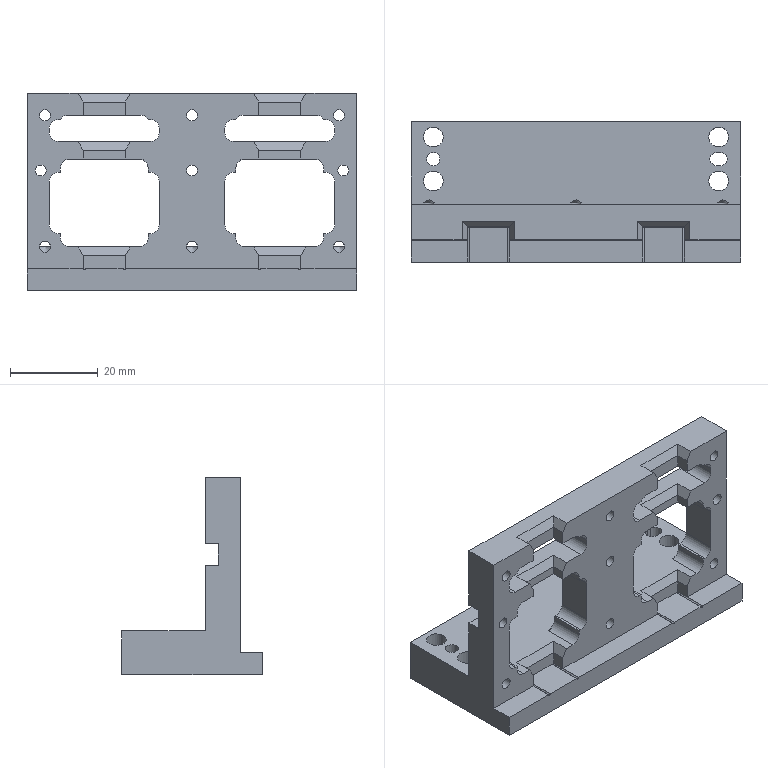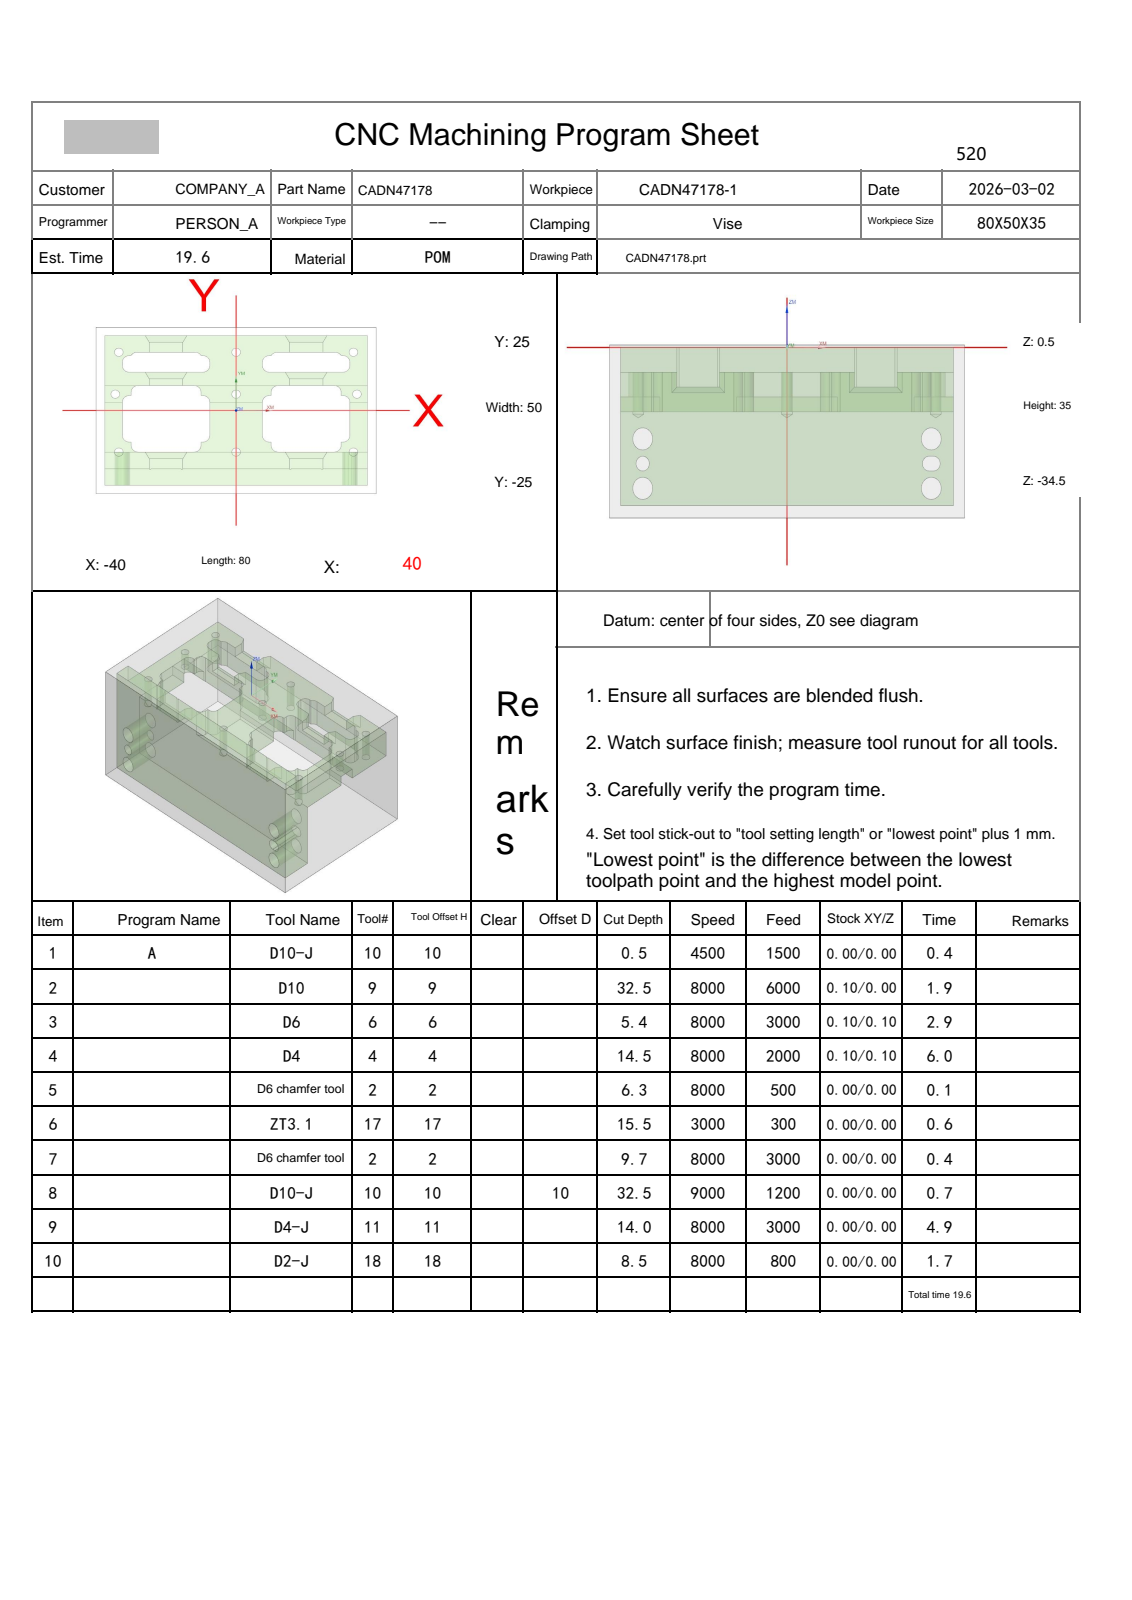NC program | NX | posted by the shop | part box 75 x 32 x 45 mm
Lines 1489 to 2470 of 18359:
N4 T04 M06
(D4  D=4. R=0. H=04 ce=0.10 di=0.10)
G00 G90 G54 X-22.782 Y27.43 M03 S8000
G43 H04 Z10.5
M08
Z-4.3
G01 Z-5.5 F2000.
G03 X-19.982 Y24.63 I2.8 J0.0
G01 X-14.557
X-14.478 Y24.64
X-14.477 Y24.561
G03 X-15.908 Y23.475 I.415 J-2.031
G01 X-17.081 Y21.442
X-17.111 Y21.371
G03 X-17.3 Y20.529 I1.911 J-.872
G01 Y17.38
G03 X-16.933 Y16.314 I2.104 J.128
X-15.2 Y15.4 I1.733 J1.186
G01 X-11.789
G03 X-10.586 Y14.484 I1.789 J1.1
X-9.909 Y14.379 I.678 J2.135
X-9.6 Y14.4 I0.0 J2.24
G01 Y13.6
X-14.181
G03 X-15.875 Y12.531 I.079 J-2.001
G01 X-17.019 Y10.55
G03 X-17.3 Y9.686 I1.471 J-.957
G01 Y7.286
G03 X-16.859 Y6.212 I2.113 J.241
X-15.936 Y5.533 I1.659 J1.288
X-15.277 Y5.402 I.735 J1.967
G01 X-15.17 Y5.4
X-12.108
X-12.1 Y5.375
Y4.5
G03 X-11.234 Y2.801 I2.1 J0.0
X-10.193 Y2.4 I1.256 J1.709
G01 X-9.6
Y-7.4
X-9.605
G03 X-9.907 Y-7.379 I-.302 J-2.202
X-10.509 Y-7.463 I0.0 J-2.223
X-12.091 Y-9.307 I.509 J-2.037
X-12.136 Y-9.884 I3.719 J-.576
X-12.1 Y-10.4 I3.764 J0.0
G01 X-14.045
G03 X-15.864 Y-11.45 I0.0 J-2.1
G01 X-16.673 Y-12.852
X-17.08 Y-13.557
G03 X-17.301 Y-14.438 I1.65 J-.882
G01 X-17.3 Y-14.5
Y-15.4
X-22.7
Y-14.5
X-22.697 Y-14.395
G03 X-22.876 Y-13.632 I-1.711 J0.0
G01 X-23.51 Y-12.535
X-24.14 Y-11.443
G03 X-25.21 Y-10.536 I-1.815 J-1.057
X-25.76 Y-10.4 I-.794 J-2.021
G01 X-25.976
X-27.9 Y-10.398
G03 X-27.867 Y-9.892 I-3.867 J.506
X-27.906 Y-9.342 I-3.9 J0.0
X-29.442 Y-7.475 I-2.094 J-.158
X-30.091 Y-7.378 I-.649 J-2.122
X-30.4 Y-7.4 I0.0 J-2.219
G01 Y2.4
X-29.751
G03 X-28.37 Y3.176 I-.262 J2.083
X-27.9 Y4.5 I-1.63 J1.324
G01 Y5.4
X-24.851
X-24.651 Y5.405
G03 X-23.152 Y6.199 I-.149 J2.095
X-22.891 Y6.616 I-1.662 J1.328
G02 X-22.53 Y6.844 I.361 J-.171
X-22.3 Y6.772 I0.0 J-.4
G01 X-20.633 Y5.607
G03 X-20.404 Y5.535 I.229 J.328
X-20.202 Y5.589 I0.0 J.4
G02 X-20. Y5.644 I.202 J-.345
X-19.639 Y5.416 I0.0 J-.4
G03 X-19.066 Y4.489 I4.452 J2.11
X-15.364 Y2.603 I3.865 J3.011
G01 X-15.187 Y2.6
X-15.161
X-14.774
G02 X-14.415 Y2.374 I-.001 J-.4
G03 X-12.887 Y.54 I4.415 J2.126
X-12.587 Y.338 I2.908 J3.97
G02 X-12.4 Y0.0 I-.213 J-.339
G01 Y-5.001
G02 X-12.588 Y-5.339 I-.4 J.001
G03 X-14.439 Y-7.424 I2.588 J-4.161
G02 X-14.743 Y-7.65 I-.362 J.17
G03 X-18.289 Y-10.05 I.698 J-4.85
G01 X-19.622 Y-12.377
G02 X-19.982 Y-12.601 I-.36 J.177
G01 X-20.015 Y-12.6
G02 X-20.372 Y-12.379 I.001 J.4
G01 X-20.408 Y-12.307
X-21.72 Y-10.034
G03 X-24.202 Y-7.924 I-4.234 J-2.466
X-25.263 Y-7.642 I-1.802 J-4.634
G02 X-25.565 Y-7.417 I.06 J.395
G03 X-27.412 Y-5.339 I-4.435 J-2.083
G02 X-27.6 Y-5.001 I.212 J.339
G01 Y-.007
G02 X-27.413 Y.33 I.4 J-.001
G03 X-26.618 Y.95 I-2.6 J4.153
X-26.152 Y1.466 I-3.394 J3.534
X-25.585 Y2.374 I-3.848 J3.034
G02 X-25.226 Y2.6 I.36 J-.174
G01 X-24.87
X-24.814
G03 X-24.531 Y2.608 I0.0 J4.928
X-21.114 Y4.272 I-.269 J4.893
G02 X-20.933 Y4.354 I.18 J-.158
X-20.716 Y4.215 I0.0 J-.24
G01 X-19.222 Y1.014
G03 X-19.06 Y.837 I.362 J.169
X-16.302 Y-.12 I3.859 J6.663
G02 X-16.046 Y-.268 I-.058 J-.396
G03 X-15.323 Y-1.064 I6.046 J4.768
G02 X-15.2 Y-1.351 I-.277 J-.288
G01 Y-3.667
G02 X-15.323 Y-3.936 I-.4 J.02
G03 X-16.283 Y-5.048 I5.323 J-5.564
G02 X-16.481 Y-5.195 I-.326 J.232
G03 X-19.707 Y-7.281 I2.436 J-7.305
G02 X-20. Y-7.409 I-.293 J.272
X-20.293 Y-7.281 I0.0 J.4
G03 X-23.194 Y-5.312 I-5.661 J-5.219
X-23.521 Y-5.193 I-2.81 J-7.246
G02 X-23.718 Y-5.047 I.129 J.379
G03 X-24.677 Y-3.936 I-6.282 J-4.453
G02 X-24.8 Y-3.649 I.277 J.288
G01 Y-1.341
G02 X-24.678 Y-1.068 I.4 J-.015
G03 X-24.007 Y-.334 I-5.335 J5.552
G01 X-23.954 Y-.268
G02 X-23.698 Y-.12 I.314 J-.248
G03 X-21.222 Y.682 I-1.101 J7.621
G01 X-21.036 Y.728
G02 X-20.69 Y.528 I0.0 J-.4
G01 X-19.15 Y-2.135
G03 X-18.947 Y-2.309 I.346 J.2
G01 X-18.776 Y-2.372
G02 X-18.514 Y-2.748 I-.137 J-.376
X-18.734 Y-3.105 I-.4 J0.0
G03 X-19.782 Y-3.706 I4.689 J-9.395
G02 X-20. Y-3.77 I-.218 J.336
X-20.218 Y-3.706 I0.0 J.4
G03 X-21.266 Y-3.105 I-5.737 J-8.794
G02 X-21.486 Y-2.748 I.18 J.357
X-21.224 Y-2.372 I.4 J0.0
G01 X-21.125 Y-2.336
G03 X-20.877 Y-2.057 I-.14 J.375
G01 X-20.048 Y1.311
X-20.038 Y1.439
X-20.339 Y5.14
G03 X-20.628 Y5.492 I-.399 J-.033
G01 X-22.638 Y6.06
G02 X-22.93 Y6.444 I.109 J.385
G01 X-22.891 Y6.616
G03 X-22.736 Y7.068 I-1.922 J.911
G02 X-22.401 Y7.378 I.391 J-.086
G01 X-21.345 Y7.525
G03 X-21. Y7.921 I-.055 J.396
G01 Y10.327
G02 X-20. Y11.327 I1. J0.0
X-19. Y10.327 I0.0 J-1.
G01 Y6.684
G02 X-20. Y5.684 I-1. J0.0
X-20.591 Y5.877 I0.0 J1.
G01 X-20.685 Y5.929
X-22.487 Y6.607
G02 X-22.746 Y6.982 I.141 J.374
G01 X-22.736 Y7.068
G03 X-22.7 Y7.284 I-2.077 J.459
G01 Y9.688
G03 X-22.981 Y10.55 I-1.749 J-.094
G01 X-23.877 Y12.101
X-24.136 Y12.55
G03 X-24.611 Y13.114 I-1.819 J-1.05
X-25.762 Y13.6 I-1.369 J-1.635
G01 X-30.4
X-30.396 Y14.4
G03 X-30.095 Y14.38 I.301 J2.23
X-29.486 Y14.464 I0.0 J2.25
X-28.211 Y15.4 I-.514 J2.036
G01 X-24.71 Y15.402
G03 X-23.007 Y16.408 I-.09 J2.098
X-22.7 Y17.377 I-1.799 J1.102
G01 Y20.535
X-22.699 Y20.605
G03 X-22.894 Y21.399 I-1.71 J0.0
G01 X-24.03 Y23.367
X-24.103 Y23.492
X-24.148 Y23.57
G03 X-25.247 Y24.477 I-1.807 J-1.07
X-25.487 Y24.551 I-.753 J-2.032
G01 X-25.492 Y24.635
X-25.407 Y24.63
X-21.594
X-21.558 Y24.615
X-21.523 Y24.58
X-21.472 Y24.557
G02 X-20.569 Y23.811 I-.065 J-.998
G01 X-18.79 Y16.974
G02 X-18.758 Y16.722 I-.968 J-.252
X-19.758 Y15.722 I-1. J0.0
X-20.726 Y16.47 I0.0 J1.
G01 X-22.505 Y23.307
G02 X-22.537 Y23.559 I.968 J.252
X-21.592 Y24.558 I1. J0.0
G01 X-21.559 Y24.572
X-21.526 Y24.606
X-21.468 Y24.63
X-21.321
G02 X-20.927 Y24.296 I0.0 J-.4
G01 X-19.391 Y15.018
X-19.334 Y14.868
X-19.242 Y14.73
G03 X-18.615 Y13.987 I4.042 J2.77
G02 X-18.495 Y13.7 I-.279 J-.286
X-18.548 Y13.501 I-.4 J0.0
G01 X-19.415 Y11.999
G03 X-19.641 Y11.591 I3.868 J-2.406
G02 X-20. Y11.367 I-.359 J.176
X-20.359 Y11.591 I0.0 J.4
G03 X-20.585 Y12. I-4.09 J-1.997
G01 X-21.452 Y13.501
G02 X-21.505 Y13.7 I.347 J.199
X-21.385 Y13.987 I.4 J0.0
G03 X-20.617 Y14.948 I-3.415 J3.513
X-20.362 Y15.422 I-4.188 J2.562
G02 X-20. Y15.651 I.362 J-.171
X-19.617 Y15.378 I0.0 J-.403
G03 X-17.095 Y13.793 I2.522 J1.215
X-15.88 Y14.071 I0.0 J2.8
G01 Z-4.3
G00 Z-2.
G01 X-22.782 Y27.43 F6000.
G00 Z-4.8
G01 Z-6. F2000.
G03 X-19.982 Y24.63 I2.8 J0.0
G01 X-14.557
X-14.478 Y24.64
X-14.477 Y24.561
G03 X-15.908 Y23.475 I.415 J-2.031
G01 X-17.081 Y21.442
X-17.111 Y21.371
G03 X-17.3 Y20.5 I1.911 J-.871
G01 Y17.38
G03 X-16.933 Y16.314 I2.104 J.128
X-15.2 Y15.4 I1.733 J1.186
G01 X-11.789
G03 X-10.586 Y14.484 I1.789 J1.1
X-9.909 Y14.379 I.678 J2.135
X-9.6 Y14.4 I0.0 J2.24
G01 Y13.6
X-14.181
G03 X-15.875 Y12.531 I.079 J-2.001
G01 X-17.019 Y10.55
G03 X-17.3 Y9.686 I1.471 J-.957
G01 Y9.5
Y7.286
G03 X-16.859 Y6.212 I2.113 J.241
X-15.936 Y5.533 I1.659 J1.288
X-15.263 Y5.401 I.735 J1.967
G01 X-15.17 Y5.4
X-12.108
X-12.1 Y5.375
Y4.5
G03 X-11.234 Y2.801 I2.1 J0.0
X-10.193 Y2.4 I1.256 J1.709
G01 X-10.
X-9.6
Y-7.4
X-9.605
G03 X-9.907 Y-7.379 I-.302 J-2.202
X-10.509 Y-7.463 I0.0 J-2.223
X-12.091 Y-9.307 I.509 J-2.037
X-12.136 Y-9.884 I3.719 J-.576
X-12.1 Y-10.4 I3.764 J0.0
G01 X-14.045
G03 X-15.864 Y-11.45 I0.0 J-2.1
G01 X-17.08 Y-13.557
G03 X-17.301 Y-14.438 I1.65 J-.882
G01 X-17.3 Y-14.5
Y-15.4
X-22.7
Y-14.5
X-22.697 Y-14.395
G03 X-22.876 Y-13.632 I-1.711 J0.0
G01 X-22.981 Y-13.45
X-24.136 Y-11.45
G03 X-25.21 Y-10.536 I-1.819 J-1.05
X-25.76 Y-10.4 I-.794 J-2.021
G01 X-25.976
X-27.9 Y-10.398
G03 X-27.867 Y-9.892 I-3.867 J.506
X-27.906 Y-9.342 I-3.9 J0.0
X-29.442 Y-7.475 I-2.094 J-.158
X-30.091 Y-7.378 I-.649 J-2.122
X-30.4 Y-7.4 I0.0 J-2.219
G01 Y2.4
X-30.
X-29.751
G03 X-28.37 Y3.176 I-.262 J2.083
X-27.9 Y4.5 I-1.63 J1.324
G01 Y5.4
X-24.85
X-24.651 Y5.405
G03 X-23.152 Y6.199 I-.149 J2.095
X-22.891 Y6.616 I-1.662 J1.328
G02 X-22.53 Y6.845 I.361 J-.171
X-22.3 Y6.772 I0.0 J-.4
G01 X-20.633 Y5.607
G03 X-20.404 Y5.535 I.229 J.328
X-20.202 Y5.589 I0.0 J.4
G02 X-20. Y5.644 I.202 J-.345
X-19.639 Y5.417 I0.0 J-.4
G03 X-19.066 Y4.489 I4.452 J2.11
X-15.2 Y2.6 I3.866 J3.011
G01 X-15.189
X-14.774
G02 X-14.415 Y2.374 I-.001 J-.4
G03 X-12.887 Y.54 I4.415 J2.126
X-12.587 Y.338 I2.908 J3.97
G02 X-12.4 Y0.0 I-.213 J-.339
G01 Y-5.001
G02 X-12.588 Y-5.339 I-.4 J.001
G03 X-14.439 Y-7.424 I2.588 J-4.161
G02 X-14.743 Y-7.65 I-.362 J.17
G03 X-18.289 Y-10.05 I.697 J-4.85
G01 X-19.622 Y-12.377
G02 X-19.982 Y-12.601 I-.36 J.178
G01 X-20.016 Y-12.6
G02 X-20.372 Y-12.379 I.001 J.4
G01 X-20.408 Y-12.307
X-21.711 Y-10.05
G03 X-24.202 Y-7.924 I-4.244 J-2.45
X-25.264 Y-7.642 I-1.802 J-4.634
G02 X-25.565 Y-7.417 I.061 J.395
G03 X-27.412 Y-5.339 I-4.435 J-2.083
G02 X-27.6 Y-5.001 I.212 J.339
G01 Y-.007
G02 X-27.413 Y.33 I.4 J-.001
G03 X-26.618 Y.95 I-2.6 J4.153
X-26.152 Y1.466 I-3.394 J3.534
X-25.585 Y2.374 I-3.848 J3.034
G02 X-25.226 Y2.6 I.36 J-.174
G01 X-24.814
X-24.8
G03 X-21.114 Y4.272 I0.0 J4.9
G02 X-20.933 Y4.354 I.18 J-.158
X-20.716 Y4.215 I0.0 J-.24
G01 X-19.222 Y1.014
G03 X-19.06 Y.837 I.362 J.169
X-16.301 Y-.121 I3.86 J6.663
G02 X-16.046 Y-.268 I-.058 J-.396
G03 X-15.323 Y-1.064 I6.046 J4.768
G02 X-15.2 Y-1.351 I-.277 J-.288
G01 X-15.201 Y-3.668
G02 X-15.323 Y-3.936 I-.399 J.02
G03 X-16.283 Y-5.048 I5.323 J-5.564
G02 X-16.481 Y-5.195 I-.326 J.232
G03 X-19.707 Y-7.281 I2.436 J-7.305
G02 X-20. Y-7.409 I-.293 J.272
X-20.293 Y-7.281 I0.0 J.4
G03 X-23.194 Y-5.312 I-5.661 J-5.219
X-23.521 Y-5.193 I-2.81 J-7.246
G02 X-23.718 Y-5.047 I.129 J.379
G03 X-24.677 Y-3.936 I-6.282 J-4.453
G02 X-24.8 Y-3.649 I.277 J.288
G01 Y-1.341
G02 X-24.678 Y-1.068 I.4 J-.015
G03 X-24.007 Y-.334 I-5.335 J5.552
G01 X-23.954 Y-.268
G02 X-23.699 Y-.121 I.313 J-.249
G03 X-21.222 Y.682 I-1.101 J7.621
G01 X-21.036 Y.728
G02 X-20.69 Y.528 I0.0 J-.4
G01 X-19.15 Y-2.136
G03 X-18.947 Y-2.309 I.346 J.2
G01 X-18.777 Y-2.372
G02 X-18.514 Y-2.748 I-.137 J-.376
X-18.734 Y-3.105 I-.4 J0.0
G03 X-19.782 Y-3.706 I4.689 J-9.395
G02 X-20. Y-3.77 I-.218 J.336
X-20.218 Y-3.706 I0.0 J.4
G03 X-21.266 Y-3.105 I-5.737 J-8.794
G02 X-21.486 Y-2.748 I.18 J.357
X-21.223 Y-2.372 I.4 J0.0
G01 X-21.125 Y-2.336
G03 X-20.877 Y-2.057 I-.14 J.375
G01 X-20.048 Y1.311
X-20.038 Y1.439
X-20.338 Y5.14
G03 X-20.628 Y5.492 I-.399 J-.033
G01 X-22.638 Y6.06
G02 X-22.93 Y6.445 I.109 J.385
G01 X-22.891 Y6.616
G03 X-22.736 Y7.068 I-1.922 J.911
G02 X-22.401 Y7.378 I.391 J-.086
G01 X-21.345 Y7.525
G03 X-21. Y7.921 I-.055 J.396
G01 Y10.327
G02 X-20. Y11.327 I1. J0.0
X-19. Y10.327 I0.0 J-1.
G01 Y6.684
G02 X-20. Y5.684 I-1. J0.0
X-20.591 Y5.877 I0.0 J1.
G01 X-20.685 Y5.929
X-22.487 Y6.607
G02 X-22.746 Y6.982 I.141 J.374
G01 X-22.736 Y7.068
G03 X-22.7 Y7.284 I-2.077 J.459
G01 Y7.5
Y9.688
G03 X-22.981 Y10.55 I-1.749 J-.094
G01 X-24.136 Y12.55
G03 X-24.611 Y13.114 I-1.819 J-1.05
X-25.762 Y13.6 I-1.369 J-1.635
G01 X-25.976
X-30.4
X-30.396 Y14.4
G03 X-30.095 Y14.38 I.301 J2.23
X-29.486 Y14.464 I0.0 J2.25
X-28.211 Y15.4 I-.514 J2.036
G01 X-24.71 Y15.402
G03 X-23.007 Y16.408 I-.09 J2.098
X-22.7 Y17.377 I-1.799 J1.102
G01 Y17.5
Y20.535
X-22.699 Y20.605
G03 X-22.894 Y21.399 I-1.71 J0.0
G01 X-24.136 Y23.55
G03 X-25.247 Y24.477 I-1.819 J-1.05
X-25.487 Y24.551 I-.753 J-2.032
G01 X-25.492 Y24.635
X-25.407 Y24.63
X-21.594
X-21.558 Y24.615
X-21.523 Y24.58
X-21.472 Y24.557
G02 X-20.569 Y23.811 I-.065 J-.998
G01 X-18.79 Y16.974
G02 X-18.758 Y16.722 I-.968 J-.252
X-19.758 Y15.722 I-1. J0.0
X-20.726 Y16.47 I0.0 J1.
G01 X-22.505 Y23.307
G02 X-22.537 Y23.559 I.968 J.252
X-21.592 Y24.558 I1. J0.0
G01 X-21.559 Y24.572
X-21.526 Y24.606
X-21.468 Y24.63
X-21.321
G02 X-20.927 Y24.296 I0.0 J-.4
G01 X-19.391 Y15.018
X-19.334 Y14.868
X-19.242 Y14.73
G03 X-18.615 Y13.986 I4.042 J2.77
G02 X-18.495 Y13.7 I-.28 J-.286
X-18.548 Y13.501 I-.4 J0.0
G01 X-19.415 Y11.999
G03 X-19.641 Y11.591 I3.868 J-2.406
G02 X-20. Y11.367 I-.359 J.176
X-20.359 Y11.591 I0.0 J.4
G03 X-20.585 Y12. I-4.09 J-1.997
G01 X-21.452 Y13.501
G02 X-21.505 Y13.7 I.347 J.199
X-21.385 Y13.986 I.4 J0.0
G03 X-20.617 Y14.948 I-3.415 J3.514
X-20.362 Y15.422 I-4.188 J2.562
G02 X-20. Y15.651 I.362 J-.171
X-19.617 Y15.378 I0.0 J-.403
G03 X-17.095 Y13.793 I2.522 J1.215
X-15.88 Y14.071 I0.0 J2.8
G01 Z-4.8
G00 Z-2.5
G01 X-22.782 Y27.43 F6000.
G00 Z-5.3
G01 Z-6.5 F2000.
G03 X-19.982 Y24.63 I2.8 J0.0
G01 X-14.557
X-14.478 Y24.64
X-14.477 Y24.561
G03 X-15.908 Y23.475 I.415 J-2.031
G01 X-17.081 Y21.442
X-17.111 Y21.371
G03 X-17.3 Y20.5 I1.911 J-.871
G01 Y17.38
G03 X-16.933 Y16.314 I2.104 J.128
X-15.2 Y15.4 I1.733 J1.186
G01 X-11.789
G03 X-10.586 Y14.484 I1.789 J1.1
X-9.909 Y14.379 I.678 J2.135
X-9.6 Y14.4 I0.0 J2.24
G01 Y13.6
X-14.181
G03 X-15.875 Y12.531 I.079 J-2.001
G01 X-17.019 Y10.55
G03 X-17.3 Y9.686 I1.471 J-.957
G01 Y9.5
Y7.286
G03 X-16.859 Y6.212 I2.113 J.241
X-15.2 Y5.4 I1.659 J1.288
G01 X-12.108
X-12.1 Y5.375
Y4.5
G03 X-11.234 Y2.801 I2.1 J0.0
X-10.193 Y2.4 I1.256 J1.709
G01 X-10.
X-9.6
Y-7.4
X-9.605
G03 X-9.907 Y-7.379 I-.302 J-2.202
X-10.509 Y-7.463 I0.0 J-2.223
X-12.091 Y-9.307 I.509 J-2.037
X-12.136 Y-9.884 I3.719 J-.576
X-12.1 Y-10.4 I3.764 J0.0
G01 X-14.045
G03 X-15.864 Y-11.45 I0.0 J-2.1
G01 X-16.528 Y-12.6
X-17.019 Y-13.451
X-17.08 Y-13.557
G03 X-17.301 Y-14.438 I1.65 J-.882
G01 X-17.3 Y-14.5
Y-15.4
X-22.7
Y-14.5
X-22.697 Y-14.395
G03 X-22.876 Y-13.632 I-1.711 J0.0
G01 X-22.981 Y-13.45
X-24.136 Y-11.45
G03 X-25.21 Y-10.536 I-1.819 J-1.05
X-25.76 Y-10.4 I-.794 J-2.021
G01 X-25.976
X-27.9 Y-10.398
G03 X-27.867 Y-9.892 I-3.867 J.506
X-27.906 Y-9.342 I-3.9 J0.0
X-29.442 Y-7.475 I-2.094 J-.158
X-30.091 Y-7.378 I-.649 J-2.122
X-30.4 Y-7.4 I0.0 J-2.219
G01 Y2.4
X-29.999
X-29.751
G03 X-28.37 Y3.176 I-.262 J2.083
X-27.9 Y4.5 I-1.63 J1.324
G01 Y5.4
X-24.8
X-24.651 Y5.405
G03 X-23.152 Y6.199 I-.149 J2.095
X-22.891 Y6.616 I-1.662 J1.328
G02 X-22.53 Y6.845 I.361 J-.171
X-22.3 Y6.772 I0.0 J-.4
G01 X-20.633 Y5.607
G03 X-20.404 Y5.535 I.229 J.328
X-20.202 Y5.59 I0.0 J.4
G02 X-20. Y5.644 I.202 J-.345
X-19.639 Y5.417 I0.0 J-.4
G03 X-19.066 Y4.489 I4.452 J2.11
X-15.224 Y2.6 I3.866 J3.011
G01 X-14.774
G02 X-14.415 Y2.375 I-.001 J-.4
G03 X-12.887 Y.54 I4.415 J2.125
X-12.587 Y.337 I2.908 J3.97
G02 X-12.4 Y0.0 I-.213 J-.339
G01 Y-5.001
G02 X-12.588 Y-5.339 I-.4 J.001
G03 X-14.439 Y-7.425 I2.588 J-4.161
G02 X-14.743 Y-7.65 I-.362 J.17
G03 X-18.289 Y-10.05 I.697 J-4.85
G01 X-19.622 Y-12.378
G02 X-19.982 Y-12.601 I-.36 J.178
G01 X-20.016 Y-12.6
G02 X-20.372 Y-12.379 I.001 J.4
G01 X-20.408 Y-12.307
X-21.711 Y-10.05
G03 X-24.202 Y-7.924 I-4.244 J-2.45
X-25.264 Y-7.642 I-1.802 J-4.634
G02 X-25.565 Y-7.417 I.061 J.395
G03 X-27.412 Y-5.339 I-4.435 J-2.083
G02 X-27.6 Y-5.001 I.212 J.339
G01 Y-.007
G02 X-27.413 Y.33 I.4 J-.001
G03 X-26.618 Y.95 I-2.6 J4.153
X-26.153 Y1.466 I-3.394 J3.534
X-25.585 Y2.375 I-3.847 J3.034
G02 X-25.226 Y2.6 I.36 J-.175
G01 X-24.75
G03 X-21.114 Y4.272 I-.05 J4.9
G02 X-20.933 Y4.354 I.18 J-.158
X-20.716 Y4.215 I0.0 J-.24
G01 X-19.221 Y1.014
G03 X-19.06 Y.837 I.362 J.169
X-16.301 Y-.121 I3.86 J6.663
G02 X-16.046 Y-.268 I-.058 J-.396
G03 X-15.323 Y-1.064 I6.046 J4.768
G02 X-15.2 Y-1.351 I-.277 J-.288
G01 X-15.201 Y-3.668
G02 X-15.323 Y-3.936 I-.399 J.02
G03 X-16.283 Y-5.049 I5.323 J-5.564
G02 X-16.481 Y-5.195 I-.326 J.232
G03 X-19.707 Y-7.281 I2.436 J-7.305
G02 X-20. Y-7.409 I-.293 J.272
X-20.293 Y-7.281 I0.0 J.4
G03 X-23.194 Y-5.312 I-5.661 J-5.219
X-23.522 Y-5.193 I-2.81 J-7.246
G02 X-23.718 Y-5.047 I.129 J.379
G03 X-24.677 Y-3.936 I-6.282 J-4.453
G02 X-24.8 Y-3.649 I.277 J.288
G01 Y-1.341
G02 X-24.678 Y-1.069 I.4 J-.015
G03 X-24.007 Y-.334 I-5.335 J5.552
G01 X-23.954 Y-.268
G02 X-23.699 Y-.121 I.313 J-.249
G03 X-21.222 Y.682 I-1.101 J7.621
G01 X-21.036 Y.728
G02 X-20.69 Y.528 I0.0 J-.4
G01 X-19.15 Y-2.136
G03 X-18.947 Y-2.309 I.346 J.2
G01 X-18.777 Y-2.372
G02 X-18.514 Y-2.748 I-.137 J-.376
X-18.734 Y-3.105 I-.4 J0.0
G03 X-19.783 Y-3.706 I4.689 J-9.395
G02 X-20. Y-3.77 I-.217 J.336
X-20.217 Y-3.706 I0.0 J.4
G03 X-21.266 Y-3.105 I-5.737 J-8.794
G02 X-21.486 Y-2.748 I.18 J.357
X-21.223 Y-2.372 I.4 J0.0
G01 X-21.125 Y-2.336
G03 X-20.877 Y-2.057 I-.14 J.375
G01 X-20.048 Y1.311
X-20.038 Y1.439
X-20.338 Y5.14
G03 X-20.628 Y5.492 I-.399 J-.033
G01 X-22.638 Y6.06
G02 X-22.93 Y6.445 I.109 J.385
G01 X-22.891 Y6.616
G03 X-22.736 Y7.068 I-1.922 J.911
G02 X-22.401 Y7.378 I.391 J-.086
G01 X-21.345 Y7.525
G03 X-21. Y7.921 I-.055 J.396
G01 Y10.327
G02 X-20. Y11.327 I1. J0.0
X-19. Y10.327 I0.0 J-1.
G01 Y6.684
G02 X-20. Y5.684 I-1. J0.0
X-20.591 Y5.877 I0.0 J1.
G01 X-20.685 Y5.929
X-22.487 Y6.607
G02 X-22.746 Y6.982 I.141 J.374
G01 X-22.736 Y7.068
G03 X-22.7 Y7.284 I-2.077 J.459
G01 Y7.5
Y9.688
G03 X-22.981 Y10.55 I-1.749 J-.094
G01 X-24.136 Y12.55
G03 X-24.611 Y13.114 I-1.819 J-1.05
X-25.762 Y13.6 I-1.369 J-1.635
G01 X-25.976
X-30.4
X-30.396 Y14.4
G03 X-30.095 Y14.38 I.301 J2.23
X-29.486 Y14.464 I0.0 J2.25
X-28.211 Y15.4 I-.514 J2.036
G01 X-24.71 Y15.402
G03 X-23.007 Y16.408 I-.09 J2.098
X-22.7 Y17.377 I-1.799 J1.102
G01 Y17.5
Y20.535
X-22.699 Y20.605
G03 X-22.894 Y21.399 I-1.71 J0.0
G01 X-22.981 Y21.55
X-24.136 Y23.55
G03 X-25.247 Y24.477 I-1.819 J-1.05
X-25.487 Y24.551 I-.753 J-2.032
G01 X-25.492 Y24.635
X-25.407 Y24.63
X-21.594
X-21.558 Y24.615
X-21.523 Y24.58
X-21.472 Y24.557
G02 X-20.569 Y23.811 I-.065 J-.998
G01 X-18.79 Y16.974
G02 X-18.758 Y16.722 I-.968 J-.252
X-19.758 Y15.722 I-1. J0.0
X-20.726 Y16.47 I0.0 J1.
G01 X-22.505 Y23.307
G02 X-22.537 Y23.559 I.968 J.252
X-21.592 Y24.558 I1. J0.0
G01 X-21.559 Y24.572
X-21.526 Y24.606
X-21.468 Y24.63
X-21.321
G02 X-20.927 Y24.296 I0.0 J-.4
G01 X-19.391 Y15.018
X-19.334 Y14.868
X-19.242 Y14.73
G03 X-18.615 Y13.986 I4.042 J2.77
G02 X-18.495 Y13.7 I-.28 J-.286
X-18.548 Y13.501 I-.4 J0.0
G01 X-19.415 Y11.999
G03 X-19.641 Y11.591 I3.868 J-2.406
G02 X-20. Y11.367 I-.359 J.176
X-20.359 Y11.591 I0.0 J.4
G03 X-20.585 Y12. I-4.09 J-1.997
G01 X-21.452 Y13.501
G02 X-21.505 Y13.7 I.347 J.199
X-21.385 Y13.986 I.4 J0.0
G03 X-20.617 Y14.948 I-3.415 J3.514
X-20.362 Y15.422 I-4.188 J2.562
G02 X-20. Y15.651 I.362 J-.171
X-19.617 Y15.378 I0.0 J-.403
G03 X-17.095 Y13.793 I2.522 J1.215
X-15.88 Y14.071 I0.0 J2.8
G01 Z-5.3
G00 Z-3.
G01 X-22.782 Y27.43 F6000.
G00 Z-5.8
G01 Z-7. F2000.
G03 X-19.982 Y24.63 I2.8 J0.0
G01 X-14.557
X-14.478 Y24.64
X-14.477 Y24.561
G03 X-15.908 Y23.475 I.415 J-2.031
G01 X-17.081 Y21.442
X-17.111 Y21.371
G03 X-17.3 Y20.5 I1.911 J-.871
G01 Y17.38
G03 X-16.933 Y16.314 I2.104 J.128
X-15.2 Y15.4 I1.733 J1.186
G01 X-11.789
G03 X-10.586 Y14.484 I1.789 J1.1
X-9.909 Y14.379 I.678 J2.135
X-9.6 Y14.4 I0.0 J2.24
G01 Y13.6
X-14.181
G03 X-15.875 Y12.531 I.079 J-2.001
G01 X-17.019 Y10.55
G03 X-17.3 Y9.686 I1.471 J-.957
G01 Y9.5
Y7.286
G03 X-16.859 Y6.212 I2.113 J.241
X-15.2 Y5.4 I1.659 J1.288
G01 X-12.108
X-12.1 Y5.375
Y4.5
G03 X-11.234 Y2.801 I2.1 J0.0
X-10.193 Y2.4 I1.256 J1.709
G01 X-10.
X-9.6
Y-7.4
X-9.605
G03 X-9.907 Y-7.379 I-.302 J-2.202
X-10.509 Y-7.463 I0.0 J-2.223
X-12.091 Y-9.307 I.509 J-2.037
X-12.136 Y-9.884 I3.719 J-.576
X-12.1 Y-10.4 I3.764 J0.0
G01 X-14.045
G03 X-15.864 Y-11.45 I0.0 J-2.1
G01 X-16.528 Y-12.6
X-17.019 Y-13.451
X-17.08 Y-13.557
G03 X-17.301 Y-14.438 I1.65 J-.882
G01 X-17.3 Y-14.5
Y-15.4
X-22.7
Y-14.5
X-22.697 Y-14.395
G03 X-22.876 Y-13.632 I-1.711 J0.0
G01 X-22.981 Y-13.45
X-24.136 Y-11.45
G03 X-25.21 Y-10.536 I-1.819 J-1.05
X-25.76 Y-10.4 I-.794 J-2.021
G01 X-25.976
X-27.9 Y-10.398
G03 X-27.867 Y-9.892 I-3.867 J.506
X-27.906 Y-9.342 I-3.9 J0.0
X-29.442 Y-7.475 I-2.094 J-.158
X-30.091 Y-7.378 I-.649 J-2.122
X-30.4 Y-7.4 I0.0 J-2.219
G01 Y2.4
X-29.999
X-29.751
G03 X-28.37 Y3.176 I-.262 J2.083
X-27.9 Y4.5 I-1.63 J1.324
G01 Y5.4
X-24.8
X-24.651 Y5.405
G03 X-23.152 Y6.199 I-.149 J2.095
X-22.891 Y6.616 I-1.662 J1.328
G02 X-22.53 Y6.845 I.361 J-.171
X-22.3 Y6.773 I0.0 J-.4
G01 X-20.633 Y5.607
G03 X-20.404 Y5.535 I.229 J.328
X-20.202 Y5.59 I0.0 J.4
G02 X-20. Y5.644 I.202 J-.345
X-19.639 Y5.417 I0.0 J-.4
G03 X-19.066 Y4.489 I4.452 J2.11
X-15.22 Y2.6 I3.866 J3.011
G01 X-14.774
G02 X-14.415 Y2.375 I-.001 J-.4
G03 X-12.886 Y.54 I4.415 J2.125
X-12.587 Y.337 I2.908 J3.97
G02 X-12.4 Y0.0 I-.213 J-.338
G01 Y-5.001
G02 X-12.588 Y-5.339 I-.4 J.001
G03 X-14.439 Y-7.425 I2.588 J-4.161
G02 X-14.742 Y-7.65 I-.362 J.171
G03 X-18.289 Y-10.05 I.697 J-4.85
G01 X-19.622 Y-12.378
G02 X-19.982 Y-12.601 I-.36 J.178
G01 X-20.016 Y-12.6
G02 X-20.372 Y-12.379 I.001 J.4
G01 X-20.408 Y-12.307
X-21.711 Y-10.05
G03 X-24.202 Y-7.924 I-4.244 J-2.45
X-25.264 Y-7.642 I-1.802 J-4.634
G02 X-25.565 Y-7.417 I.061 J.395
G03 X-27.412 Y-5.339 I-4.435 J-2.083
G02 X-27.6 Y-5.001 I.212 J.339
G01 Y-.007
G02 X-27.413 Y.33 I.4 J-.001
G03 X-26.618 Y.95 I-2.6 J4.153
X-26.152 Y1.466 I-3.394 J3.534
X-25.585 Y2.375 I-3.848 J3.034
G02 X-25.226 Y2.6 I.36 J-.175
G01 X-24.75
G03 X-21.113 Y4.272 I-.05 J4.9
G02 X-20.933 Y4.354 I.18 J-.158
X-20.716 Y4.215 I0.0 J-.24
G01 X-19.221 Y1.014
G03 X-19.06 Y.837 I.362 J.169
X-16.301 Y-.121 I3.86 J6.663
G02 X-16.046 Y-.268 I-.059 J-.396
G03 X-15.323 Y-1.064 I6.046 J4.768
G02 X-15.2 Y-1.351 I-.277 J-.288
G01 Y-3.668
G02 X-15.323 Y-3.936 I-.399 J.02
G03 X-16.283 Y-5.049 I5.323 J-5.564
G02 X-16.481 Y-5.195 I-.326 J.232
G03 X-19.707 Y-7.281 I2.435 J-7.305
G02 X-20. Y-7.409 I-.293 J.272
X-20.293 Y-7.281 I0.0 J.4
G03 X-23.194 Y-5.312 I-5.662 J-5.219
X-23.522 Y-5.193 I-2.81 J-7.246
G02 X-23.718 Y-5.047 I.129 J.379
G03 X-24.677 Y-3.936 I-6.282 J-4.453
G02 X-24.8 Y-3.649 I.277 J.288
G01 Y-1.341
G02 X-24.678 Y-1.069 I.4 J-.015
G03 X-24.007 Y-.334 I-5.335 J5.552
G01 X-23.954 Y-.268
G02 X-23.699 Y-.121 I.313 J-.249
G03 X-21.222 Y.682 I-1.101 J7.621
G01 X-21.036 Y.728
G02 X-20.69 Y.528 I0.0 J-.4
G01 X-19.15 Y-2.136
G03 X-18.947 Y-2.309 I.346 J.2
G01 X-18.776 Y-2.372
G02 X-18.514 Y-2.748 I-.138 J-.376
X-18.734 Y-3.105 I-.4 J0.0
G03 X-19.783 Y-3.706 I4.689 J-9.395
G02 X-20. Y-3.77 I-.217 J.336
X-20.217 Y-3.706 I0.0 J.4
G03 X-21.266 Y-3.105 I-5.737 J-8.794
G02 X-21.486 Y-2.748 I.18 J.357
X-21.223 Y-2.372 I.4 J0.0
G01 X-21.125 Y-2.336
G03 X-20.877 Y-2.057 I-.14 J.375
G01 X-20.048 Y1.311
X-20.038 Y1.439
X-20.338 Y5.14
G03 X-20.628 Y5.492 I-.399 J-.033
G01 X-22.638 Y6.06
G02 X-22.93 Y6.445 I.109 J.385
G01 X-22.891 Y6.616
G03 X-22.736 Y7.068 I-1.923 J.911
G02 X-22.401 Y7.378 I.391 J-.086
G01 X-21.345 Y7.525
G03 X-21. Y7.921 I-.055 J.396
G01 Y10.327
G02 X-20. Y11.327 I1. J0.0
X-19. Y10.327 I0.0 J-1.
G01 Y6.684
G02 X-20. Y5.684 I-1. J0.0
X-20.591 Y5.877 I0.0 J1.
G01 X-20.685 Y5.929
X-22.487 Y6.607
G02 X-22.746 Y6.982 I.141 J.374
G01 X-22.736 Y7.068
G03 X-22.7 Y7.284 I-2.077 J.459
G01 Y7.5
Y9.688
G03 X-22.981 Y10.55 I-1.749 J-.094
G01 X-24.136 Y12.55
G03 X-24.611 Y13.114 I-1.819 J-1.05
X-25.762 Y13.6 I-1.369 J-1.635
G01 X-25.976
X-30.4
X-30.396 Y14.4
G03 X-30.095 Y14.38 I.301 J2.23
X-29.486 Y14.464 I0.0 J2.25
X-28.211 Y15.4 I-.514 J2.036
G01 X-24.71 Y15.402
G03 X-23.007 Y16.408 I-.09 J2.098
X-22.7 Y17.377 I-1.799 J1.102
G01 Y17.5
Y20.535
X-22.699 Y20.605
G03 X-22.894 Y21.399 I-1.71 J0.0
G01 X-22.981 Y21.55
X-24.136 Y23.55
G03 X-25.247 Y24.477 I-1.819 J-1.05
X-25.487 Y24.551 I-.753 J-2.032
G01 X-25.492 Y24.635
X-25.407 Y24.63
X-21.594
X-21.558 Y24.615
X-21.523 Y24.58
X-21.472 Y24.557
G02 X-20.569 Y23.811 I-.065 J-.998
G01 X-18.79 Y16.974
G02 X-18.758 Y16.722 I-.968 J-.252
X-19.758 Y15.722 I-1. J0.0
X-20.726 Y16.47 I0.0 J1.
G01 X-22.505 Y23.307
G02 X-22.537 Y23.559 I.968 J.252
X-21.592 Y24.558 I1. J0.0
G01 X-21.559 Y24.572
X-21.526 Y24.606
X-21.468 Y24.63
X-21.321
G02 X-20.927 Y24.296 I0.0 J-.4
G01 X-19.391 Y15.018
X-19.334 Y14.868
X-19.242 Y14.73
G03 X-18.615 Y13.986 I4.042 J2.77
G02 X-18.495 Y13.7 I-.28 J-.286
X-18.548 Y13.501 I-.4 J0.0
G01 X-19.415 Y11.999
G03 X-19.641 Y11.591 I3.868 J-2.406
G02 X-20. Y11.367 I-.359 J.177
X-20.359 Y11.591 I0.0 J.4
G03 X-20.585 Y12. I-4.09 J-1.997
G01 X-21.452 Y13.501
G02 X-21.505 Y13.7 I.347 J.199
X-21.385 Y13.986 I.4 J0.0
G03 X-20.617 Y14.948 I-3.415 J3.514
X-20.362 Y15.422 I-4.188 J2.562
G02 X-20. Y15.651 I.361 J-.171
X-19.617 Y15.378 I0.0 J-.403
G03 X-17.095 Y13.793 I2.522 J1.215
X-15.88 Y14.071 I0.0 J2.8
G01 Z-5.8
G00 Z-3.5
G01 X-22.782 Y27.43 F6000.
G00 Z-6.3
G01 Z-7.5 F2000.
G03 X-19.982 Y24.63 I2.8 J0.0
G01 X-14.557
X-14.478 Y24.64
X-14.477 Y24.561
G03 X-15.908 Y23.475 I.415 J-2.031
G01 X-17.081 Y21.442
X-17.111 Y21.371
G03 X-17.3 Y20.5 I1.911 J-.871
G01 Y17.38
G03 X-16.933 Y16.314 I2.104 J.128
X-15.2 Y15.4 I1.733 J1.186
G01 X-11.789
G03 X-10.586 Y14.484 I1.789 J1.1
X-9.909 Y14.379 I.678 J2.135
X-9.6 Y14.4 I0.0 J2.24
G01 Y13.6
X-14.181